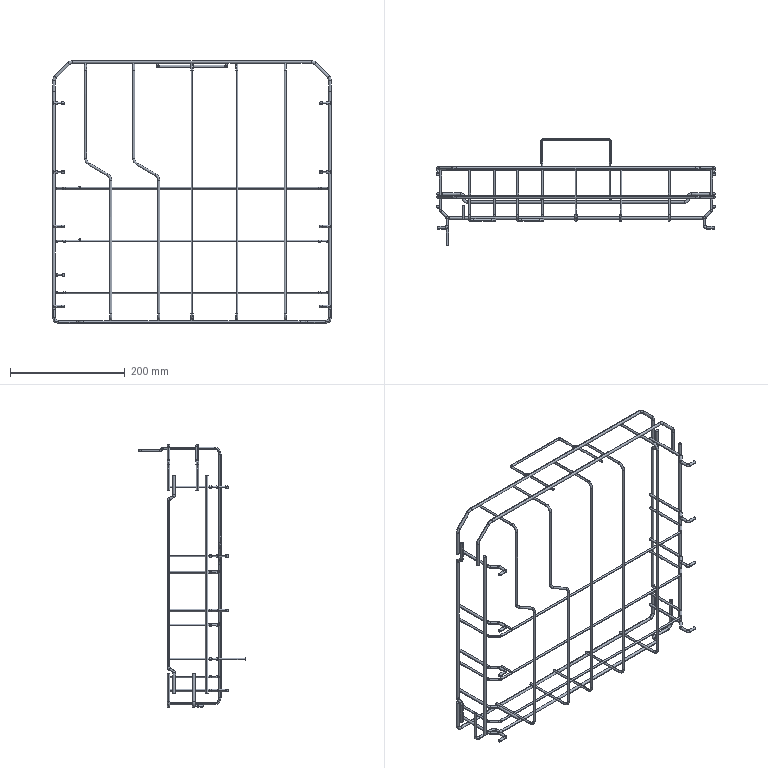Part | STEP file | ZXW722-L-178_XIAGEJIA_19_1_2_1_ | 1 solid | 440 faces | box 487 x 185.95 x 459 mm | volume 160339 mm3 | cylinder 220 | torus 164 | plane 56 | commonest cylinder face diameters 3.9 x82 4.5 x70 5 x64 2.6 x4